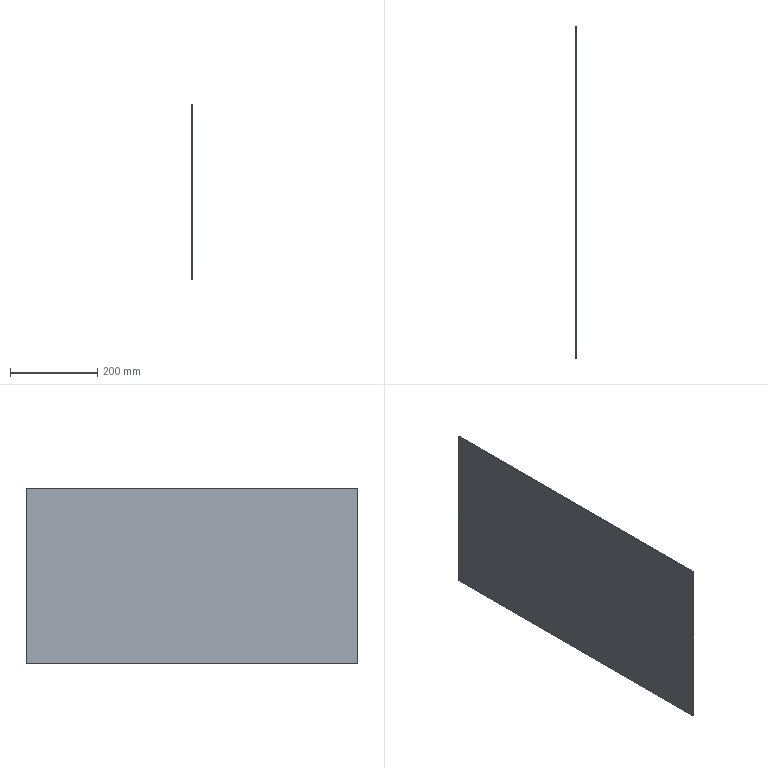Part | STEP file | Guide wheel mechanism revised.sldasm-Part-169 | 1 solid | 6 faces | box 2 x 760 x 403.01 mm | volume 612575 mm3 | plane 6
STEP:
#1=CARTESIAN_POINT('',(360.,760.,-200.));
#2=VERTEX_POINT('',#1);
#3=CARTESIAN_POINT('',(360.,0.,-200.));
#4=VERTEX_POINT('',#3);
#5=CARTESIAN_POINT('',(360.,760.,-200.));
#6=DIRECTION('',(0.,-1.,0.));
#7=VECTOR('',#6,1000.);
#8=LINE('',#5,#7);
#9=EDGE_CURVE('',#2,#4,#8,.T.);
#10=ORIENTED_EDGE('',*,*,#9,.F.);
#11=CARTESIAN_POINT('',(362.,760.,-200.));
#12=VERTEX_POINT('',#11);
#13=CARTESIAN_POINT('',(362.,760.,-200.));
#14=DIRECTION('',(-1.,0.,0.));
#15=VECTOR('',#14,1000.);
#16=LINE('',#13,#15);
#17=EDGE_CURVE('',#12,#2,#16,.T.);
#18=ORIENTED_EDGE('',*,*,#17,.F.);
#19=CARTESIAN_POINT('',(362.,0.,-200.));
#20=VERTEX_POINT('',#19);
#21=CARTESIAN_POINT('',(362.,760.,-200.));
#22=DIRECTION('',(0.,-1.,0.));
#23=VECTOR('',#22,1000.);
#24=LINE('',#21,#23);
#25=EDGE_CURVE('',#12,#20,#24,.T.);
#26=ORIENTED_EDGE('',*,*,#25,.T.);
#27=CARTESIAN_POINT('',(362.,0.,-200.));
#28=DIRECTION('',(-1.,0.,0.));
#29=VECTOR('',#28,1000.);
#30=LINE('',#27,#29);
#31=EDGE_CURVE('',#20,#4,#30,.T.);
#32=ORIENTED_EDGE('',*,*,#31,.T.);
#33=EDGE_LOOP('',(#10,#18,#26,#32));
#34=FACE_OUTER_BOUND('',#33,.T.);
#35=CARTESIAN_POINT('',(362.,760.,-200.));
#36=DIRECTION('',(0.,0.,-1.));
#37=DIRECTION('',(0.,1.,0.));
#38=AXIS2_PLACEMENT_3D('',#35,#36,#37);
#39=PLANE('',#38);
#40=ADVANCED_FACE('',(#34),#39,.T.);
#41=CARTESIAN_POINT('',(360.,760.,203.01));
#42=VERTEX_POINT('',#41);
#43=CARTESIAN_POINT('',(360.,760.,-200.));
#44=DIRECTION('',(0.,0.,-1.));
#45=VECTOR('',#44,1000.);
#46=LINE('',#43,#45);
#47=EDGE_CURVE('',#42,#2,#46,.T.);
#48=ORIENTED_EDGE('',*,*,#47,.F.);
#49=CARTESIAN_POINT('',(362.,760.,203.01));
#50=VERTEX_POINT('',#49);
#51=CARTESIAN_POINT('',(362.,760.,203.01));
#52=DIRECTION('',(-1.,0.,0.));
#53=VECTOR('',#52,1000.);
#54=LINE('',#51,#53);
#55=EDGE_CURVE('',#50,#42,#54,.T.);
#56=ORIENTED_EDGE('',*,*,#55,.F.);
#57=CARTESIAN_POINT('',(362.,760.,-200.));
#58=DIRECTION('',(0.,0.,-1.));
#59=VECTOR('',#58,1000.);
#60=LINE('',#57,#59);
#61=EDGE_CURVE('',#50,#12,#60,.T.);
#62=ORIENTED_EDGE('',*,*,#61,.T.);
#63=ORIENTED_EDGE('',*,*,#17,.T.);
#64=EDGE_LOOP('',(#48,#56,#62,#63));
#65=FACE_OUTER_BOUND('',#64,.T.);
#66=CARTESIAN_POINT('',(362.,760.,-200.));
#67=DIRECTION('',(0.,1.,0.));
#68=DIRECTION('',(0.,0.,1.));
#69=AXIS2_PLACEMENT_3D('',#66,#67,#68);
#70=PLANE('',#69);
#71=ADVANCED_FACE('',(#65),#70,.T.);
#72=CARTESIAN_POINT('',(360.,0.,203.01));
#73=VERTEX_POINT('',#72);
#74=CARTESIAN_POINT('',(360.,760.,203.01));
#75=DIRECTION('',(0.,1.,0.));
#76=VECTOR('',#75,1000.);
#77=LINE('',#74,#76);
#78=EDGE_CURVE('',#73,#42,#77,.T.);
#79=ORIENTED_EDGE('',*,*,#78,.F.);
#80=CARTESIAN_POINT('',(362.,0.,203.01));
#81=VERTEX_POINT('',#80);
#82=CARTESIAN_POINT('',(362.,0.,203.01));
#83=DIRECTION('',(-1.,0.,0.));
#84=VECTOR('',#83,1000.);
#85=LINE('',#82,#84);
#86=EDGE_CURVE('',#81,#73,#85,.T.);
#87=ORIENTED_EDGE('',*,*,#86,.F.);
#88=CARTESIAN_POINT('',(362.,760.,203.01));
#89=DIRECTION('',(0.,1.,0.));
#90=VECTOR('',#89,1000.);
#91=LINE('',#88,#90);
#92=EDGE_CURVE('',#81,#50,#91,.T.);
#93=ORIENTED_EDGE('',*,*,#92,.T.);
#94=ORIENTED_EDGE('',*,*,#55,.T.);
#95=EDGE_LOOP('',(#79,#87,#93,#94));
#96=FACE_OUTER_BOUND('',#95,.T.);
#97=CARTESIAN_POINT('',(362.,760.,203.01));
#98=DIRECTION('',(0.,0.,1.));
#99=DIRECTION('',(0.,-1.,0.));
#100=AXIS2_PLACEMENT_3D('',#97,#98,#99);
#101=PLANE('',#100);
#102=ADVANCED_FACE('',(#96),#101,.T.);
#103=CARTESIAN_POINT('',(360.,0.,-200.));
#104=DIRECTION('',(0.,0.,1.));
#105=VECTOR('',#104,1000.);
#106=LINE('',#103,#105);
#107=EDGE_CURVE('',#4,#73,#106,.T.);
#108=ORIENTED_EDGE('',*,*,#107,.F.);
#109=ORIENTED_EDGE('',*,*,#31,.F.);
#110=CARTESIAN_POINT('',(362.,0.,-200.));
#111=DIRECTION('',(0.,0.,1.));
#112=VECTOR('',#111,1000.);
#113=LINE('',#110,#112);
#114=EDGE_CURVE('',#20,#81,#113,.T.);
#115=ORIENTED_EDGE('',*,*,#114,.T.);
#116=ORIENTED_EDGE('',*,*,#86,.T.);
#117=EDGE_LOOP('',(#108,#109,#115,#116));
#118=FACE_OUTER_BOUND('',#117,.T.);
#119=CARTESIAN_POINT('',(362.,0.,-200.));
#120=DIRECTION('',(0.,-1.,0.));
#121=DIRECTION('',(0.,0.,-1.));
#122=AXIS2_PLACEMENT_3D('',#119,#120,#121);
#123=PLANE('',#122);
#124=ADVANCED_FACE('',(#118),#123,.T.);
#125=ORIENTED_EDGE('',*,*,#25,.F.);
#126=ORIENTED_EDGE('',*,*,#61,.F.);
#127=ORIENTED_EDGE('',*,*,#92,.F.);
#128=ORIENTED_EDGE('',*,*,#114,.F.);
#129=EDGE_LOOP('',(#125,#126,#127,#128));
#130=FACE_OUTER_BOUND('',#129,.T.);
#131=CARTESIAN_POINT('',(362.,0.,0.));
#132=DIRECTION('',(-1.,0.,0.));
#133=DIRECTION('',(0.,0.,1.));
#134=AXIS2_PLACEMENT_3D('',#131,#132,#133);
#135=PLANE('',#134);
#136=ADVANCED_FACE('',(#130),#135,.F.);
#137=ORIENTED_EDGE('',*,*,#9,.T.);
#138=ORIENTED_EDGE('',*,*,#107,.T.);
#139=ORIENTED_EDGE('',*,*,#78,.T.);
#140=ORIENTED_EDGE('',*,*,#47,.T.);
#141=EDGE_LOOP('',(#137,#138,#139,#140));
#142=FACE_OUTER_BOUND('',#141,.T.);
#143=CARTESIAN_POINT('',(360.,0.,0.));
#144=DIRECTION('',(-1.,0.,0.));
#145=DIRECTION('',(0.,0.,1.));
#146=AXIS2_PLACEMENT_3D('',#143,#144,#145);
#147=PLANE('',#146);
#148=ADVANCED_FACE('',(#142),#147,.T.);
#149=CLOSED_SHELL('',(#40,#71,#102,#124,#136,#148));
#150=MANIFOLD_SOLID_BREP('',#149);
#151=CARTESIAN_POINT('',(0.,0.,0.));
#152=DIRECTION('',(0.,0.,1.));
#153=DIRECTION('',(1.,0.,0.));
#154=AXIS2_PLACEMENT_3D('',#151,#152,#153);
#155=(LENGTH_UNIT()NAMED_UNIT(*)SI_UNIT(.MILLI.,.METRE.));
#156=UNCERTAINTY_MEASURE_WITH_UNIT(LENGTH_MEASURE(0.00001),#155,'','');
#157=(NAMED_UNIT(*)PLANE_ANGLE_UNIT()SI_UNIT($,.RADIAN.));
#158=(NAMED_UNIT(*)SI_UNIT($,.STERADIAN.)SOLID_ANGLE_UNIT());
#159=(GEOMETRIC_REPRESENTATION_CONTEXT(3)GLOBAL_UNCERTAINTY_ASSIGNED_CONTEXT((#156))GLOBAL_UNIT_ASSIGNED_CONTEXT((#155,#157,#158))REPRESENTATION_CONTEXT('',''));
#160=ADVANCED_BREP_SHAPE_REPRESENTATION('',(#150,#154),#159);